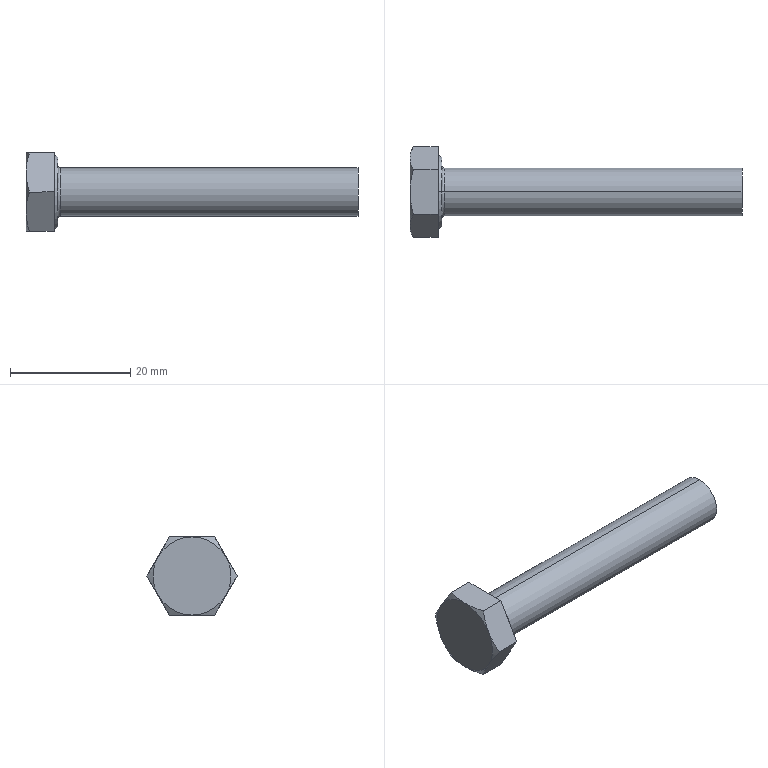Part | SolidWorks | features BaseBody 1, MoveFace 1 | 1 solid | 22 faces | box 55.3 x 15.011 x 13 mm | volume 3267 mm3 | plane 10 | cone 8 | spline 2 | cylinder 2 | commonest cylinder face diameters 8 x2
STEP:
#1=CARTESIAN_POINT('',(5.3,0.,4.4));
#2=VERTEX_POINT('',#1);
#3=CARTESIAN_POINT('',(5.3,0.,-4.4));
#4=VERTEX_POINT('',#3);
#5=CARTESIAN_POINT('',(5.3,0.,4.4));
#6=CARTESIAN_POINT('',(5.3,0.2797,4.4));
#7=CARTESIAN_POINT('',(5.3,0.6919,4.361));
#8=CARTESIAN_POINT('',(5.3,1.16,4.249));
#9=CARTESIAN_POINT('',(5.3,1.391,4.176));
#10=CARTESIAN_POINT('',(5.3,1.489,4.141));
#11=CARTESIAN_POINT('',(5.3,1.554,4.116));
#12=CARTESIAN_POINT('',(5.3,1.585,4.105));
#13=CARTESIAN_POINT('',(5.3,1.758,4.036));
#14=CARTESIAN_POINT('',(5.3,1.96,3.944));
#15=CARTESIAN_POINT('',(5.3,2.154,3.837));
#16=CARTESIAN_POINT('',(5.3,2.282,3.763));
#17=CARTESIAN_POINT('',(5.3,2.344,3.724));
#18=CARTESIAN_POINT('',(5.3,2.662,3.517));
#19=CARTESIAN_POINT('',(5.3,2.897,3.326));
#20=CARTESIAN_POINT('',(5.3,3.219,3.004));
#21=CARTESIAN_POINT('',(5.3,3.37,2.836));
#22=CARTESIAN_POINT('',(5.3,3.509,2.656));
#23=CARTESIAN_POINT('',(5.3,3.598,2.534));
#24=CARTESIAN_POINT('',(5.3,3.642,2.47));
#25=CARTESIAN_POINT('',(5.3,3.764,2.283));
#26=CARTESIAN_POINT('',(5.3,3.876,2.092));
#27=CARTESIAN_POINT('',(5.3,3.989,1.859));
#28=CARTESIAN_POINT('',(5.3,4.042,1.74));
#29=CARTESIAN_POINT('',(5.3,4.063,1.689));
#30=CARTESIAN_POINT('',(5.3,4.077,1.654));
#31=CARTESIAN_POINT('',(5.3,4.085,1.636));
#32=CARTESIAN_POINT('',(5.3,4.297,1.1));
#33=CARTESIAN_POINT('',(5.3,4.4,0.5592));
#34=CARTESIAN_POINT('',(5.3,4.4,-0.2796));
#35=CARTESIAN_POINT('',(5.3,4.361,-0.6917));
#36=CARTESIAN_POINT('',(5.3,4.249,-1.16));
#37=CARTESIAN_POINT('',(5.3,4.176,-1.391));
#38=CARTESIAN_POINT('',(5.3,4.141,-1.489));
#39=CARTESIAN_POINT('',(5.3,4.116,-1.554));
#40=CARTESIAN_POINT('',(5.3,4.105,-1.585));
#41=CARTESIAN_POINT('',(5.3,4.036,-1.758));
#42=CARTESIAN_POINT('',(5.3,3.944,-1.96));
#43=CARTESIAN_POINT('',(5.3,3.837,-2.154));
#44=CARTESIAN_POINT('',(5.3,3.763,-2.282));
#45=CARTESIAN_POINT('',(5.3,3.724,-2.344));
#46=CARTESIAN_POINT('',(5.3,3.517,-2.662));
#47=CARTESIAN_POINT('',(5.3,3.326,-2.897));
#48=CARTESIAN_POINT('',(5.3,3.004,-3.219));
#49=CARTESIAN_POINT('',(5.3,2.836,-3.37));
#50=CARTESIAN_POINT('',(5.3,2.656,-3.509));
#51=CARTESIAN_POINT('',(5.3,2.534,-3.598));
#52=CARTESIAN_POINT('',(5.3,2.47,-3.642));
#53=CARTESIAN_POINT('',(5.3,2.283,-3.764));
#54=CARTESIAN_POINT('',(5.3,2.092,-3.876));
#55=CARTESIAN_POINT('',(5.3,1.859,-3.989));
#56=CARTESIAN_POINT('',(5.3,1.74,-4.042));
#57=CARTESIAN_POINT('',(5.3,1.689,-4.063));
#58=CARTESIAN_POINT('',(5.3,1.654,-4.077));
#59=CARTESIAN_POINT('',(5.3,1.636,-4.085));
#60=CARTESIAN_POINT('',(5.3,1.1,-4.297));
#61=CARTESIAN_POINT('',(5.3,0.5597,-4.4));
#62=CARTESIAN_POINT('',(5.3,0.,-4.4));
#63=B_SPLINE_CURVE_WITH_KNOTS('',3,(#5,#6,#7,#8,#9,#10,#11,#12,#13,#14,#15,#16,#17,#18,#19,#20,#21,#22,#23,#24,#25,#26,#27,#28,#29,#30,#31,#32,#33,#34,#35,#36,#37,#38,#39,#40,#41,#42,#43,#44,#45,#46,#47,#48,#49,#50,#51,#52,#53,#54,#55,#56,#57,#58,#59,#60,#61,#62),.UNSPECIFIED.,.F.,.F.,(4,1,1,1,2,2,1,2,2,2,1,2,2,1,1,1,2,2,2,1,1,1,2,2,1,2,2,2,1,2,2,1,1,1,2,2,4),(0.,0.0625,0.09375,0.1094,0.1172,0.125,0.1563,0.1719,0.1875,0.25,0.2813,0.2969,0.3125,0.3438,0.3594,0.3672,0.3711,0.375,0.5,0.5625,0.5938,0.6094,0.6172,0.625,0.6563,0.6719,0.6875,0.75,0.7813,0.7969,0.8125,0.8438,0.8594,0.8672,0.8711,0.875,1.),.UNSPECIFIED.);
#64=EDGE_CURVE('',#2,#4,#63,.T.);
#65=ORIENTED_EDGE('',*,*,#64,.F.);
#66=CARTESIAN_POINT('',(5.7,0.,4.));
#67=VERTEX_POINT('',#66);
#68=CARTESIAN_POINT('',(5.7,0.,4.4));
#69=DIRECTION('',(0.,-1.,0.));
#70=DIRECTION('',(0.,0.,1.));
#71=AXIS2_PLACEMENT_3D('',#68,#69,#70);
#72=CIRCLE('',#71,0.4);
#73=EDGE_CURVE('',#2,#67,#72,.T.);
#74=ORIENTED_EDGE('',*,*,#73,.T.);
#75=CARTESIAN_POINT('',(5.7,0.,-4.));
#76=VERTEX_POINT('',#75);
#77=CARTESIAN_POINT('',(5.7,0.,0.));
#78=DIRECTION('',(1.,0.,0.));
#79=DIRECTION('',(0.,0.,1.));
#80=AXIS2_PLACEMENT_3D('',#77,#78,#79);
#81=CIRCLE('',#80,4.);
#82=EDGE_CURVE('',#76,#67,#81,.T.);
#83=ORIENTED_EDGE('',*,*,#82,.F.);
#84=CARTESIAN_POINT('',(5.7,0.,-4.4));
#85=DIRECTION('',(0.,1.,0.));
#86=DIRECTION('',(0.,0.,-1.));
#87=AXIS2_PLACEMENT_3D('',#84,#85,#86);
#88=CIRCLE('',#87,0.4);
#89=EDGE_CURVE('',#4,#76,#88,.T.);
#90=ORIENTED_EDGE('',*,*,#89,.F.);
#91=EDGE_LOOP('',(#65,#74,#83,#90));
#92=FACE_OUTER_BOUND('',#91,.T.);
#93=CARTESIAN_POINT('',(5.3,0.,-4.4));
#94=CARTESIAN_POINT('',(5.3,8.8,-4.4));
#95=CARTESIAN_POINT('',(5.3,8.8,4.4));
#96=CARTESIAN_POINT('',(5.3,0.,4.4));
#97=CARTESIAN_POINT('',(5.3,0.,-4.166));
#98=CARTESIAN_POINT('',(5.3,8.331,-4.166));
#99=CARTESIAN_POINT('',(5.3,8.331,4.166));
#100=CARTESIAN_POINT('',(5.3,0.,4.166));
#101=CARTESIAN_POINT('',(5.466,0.,-4.));
#102=CARTESIAN_POINT('',(5.466,8.,-4.));
#103=CARTESIAN_POINT('',(5.466,8.,4.));
#104=CARTESIAN_POINT('',(5.466,0.,4.));
#105=CARTESIAN_POINT('',(5.7,0.,-4.));
#106=CARTESIAN_POINT('',(5.7,8.,-4.));
#107=CARTESIAN_POINT('',(5.7,8.,4.));
#108=CARTESIAN_POINT('',(5.7,0.,4.));
#109=(BOUNDED_SURFACE()B_SPLINE_SURFACE(3,3,((#93,#94,#95,#96),(#97,#98,#99,#100),(#101,#102,#103,#104),(#105,#106,#107,#108)),.UNSPECIFIED.,.F.,.F.,.T.)B_SPLINE_SURFACE_WITH_KNOTS((4,4),(4,4),(0.,1.),(0.,1.),.UNSPECIFIED.)GEOMETRIC_REPRESENTATION_ITEM()RATIONAL_B_SPLINE_SURFACE(((1.,0.3333,0.3333,1.),(0.8047,0.2682,0.2682,0.8047),(0.8047,0.2682,0.2682,0.8047),(1.,0.3333,0.3333,1.)))REPRESENTATION_ITEM('')SURFACE());
#110=ADVANCED_FACE('',(#92),#109,.F.);
#111=CARTESIAN_POINT('',(55.3,0.,4.));
#112=VERTEX_POINT('',#111);
#113=CARTESIAN_POINT('',(55.3,0.,-4.));
#114=VERTEX_POINT('',#113);
#115=CARTESIAN_POINT('',(55.3,0.,0.));
#116=DIRECTION('',(-1.,0.,0.));
#117=DIRECTION('',(0.,0.,1.));
#118=AXIS2_PLACEMENT_3D('',#115,#116,#117);
#119=CIRCLE('',#118,4.);
#120=EDGE_CURVE('',#112,#114,#119,.T.);
#121=ORIENTED_EDGE('',*,*,#120,.T.);
#122=CARTESIAN_POINT('',(0.,0.,-4.));
#123=DIRECTION('',(-1.,0.,0.));
#124=VECTOR('',#123,1000.);
#125=LINE('',#122,#124);
#126=EDGE_CURVE('',#114,#76,#125,.T.);
#127=ORIENTED_EDGE('',*,*,#126,.T.);
#128=ORIENTED_EDGE('',*,*,#82,.T.);
#129=CARTESIAN_POINT('',(0.,0.,4.));
#130=DIRECTION('',(-1.,0.,0.));
#131=VECTOR('',#130,1000.);
#132=LINE('',#129,#131);
#133=EDGE_CURVE('',#112,#67,#132,.T.);
#134=ORIENTED_EDGE('',*,*,#133,.F.);
#135=EDGE_LOOP('',(#121,#127,#128,#134));
#136=FACE_OUTER_BOUND('',#135,.T.);
#137=CARTESIAN_POINT('',(0.,0.,0.));
#138=DIRECTION('',(-1.,0.,0.));
#139=DIRECTION('',(0.,0.,1.));
#140=AXIS2_PLACEMENT_3D('',#137,#138,#139);
#141=CYLINDRICAL_SURFACE('',#140,4.);
#142=ADVANCED_FACE('',(#136),#141,.T.);
#143=CARTESIAN_POINT('',(5.3,0.,-5.815));
#144=VERTEX_POINT('',#143);
#145=CARTESIAN_POINT('',(5.3,0.,5.815));
#146=VERTEX_POINT('',#145);
#147=CARTESIAN_POINT('',(5.3,0.,0.));
#148=DIRECTION('',(1.,0.,0.));
#149=DIRECTION('',(0.,0.,1.));
#150=AXIS2_PLACEMENT_3D('',#147,#148,#149);
#151=CIRCLE('',#150,5.815);
#152=EDGE_CURVE('',#144,#146,#151,.T.);
#153=ORIENTED_EDGE('',*,*,#152,.F.);
#154=CARTESIAN_POINT('',(4.7,0.,-6.161));
#155=VERTEX_POINT('',#154);
#156=CARTESIAN_POINT('',(4.7,0.,-6.161));
#157=DIRECTION('',(-0.866,0.,-0.5));
#158=VECTOR('',#157,1000.);
#159=LINE('',#156,#158);
#160=EDGE_CURVE('',#144,#155,#159,.T.);
#161=ORIENTED_EDGE('',*,*,#160,.T.);
#162=CARTESIAN_POINT('',(4.7,0.,6.161));
#163=VERTEX_POINT('',#162);
#164=CARTESIAN_POINT('',(4.7,0.,0.));
#165=DIRECTION('',(1.,0.,0.));
#166=DIRECTION('',(0.,0.,1.));
#167=AXIS2_PLACEMENT_3D('',#164,#165,#166);
#168=CIRCLE('',#167,6.161);
#169=EDGE_CURVE('',#155,#163,#168,.T.);
#170=ORIENTED_EDGE('',*,*,#169,.T.);
#171=CARTESIAN_POINT('',(4.7,0.,6.161));
#172=DIRECTION('',(-0.866,0.,0.5));
#173=VECTOR('',#172,1000.);
#174=LINE('',#171,#173);
#175=EDGE_CURVE('',#146,#163,#174,.T.);
#176=ORIENTED_EDGE('',*,*,#175,.F.);
#177=EDGE_LOOP('',(#153,#161,#170,#176));
#178=FACE_OUTER_BOUND('',#177,.T.);
#179=CARTESIAN_POINT('',(4.7,0.,0.));
#180=DIRECTION('',(-1.,0.,0.));
#181=DIRECTION('',(0.,0.,1.));
#182=AXIS2_PLACEMENT_3D('',#179,#180,#181);
#183=CONICAL_SURFACE('',#182,6.161,0.5236);
#184=ADVANCED_FACE('',(#178),#183,.T.);
#185=ORIENTED_EDGE('',*,*,#126,.F.);
#186=CARTESIAN_POINT('',(55.3,0.,0.));
#187=DIRECTION('',(-1.,0.,0.));
#188=DIRECTION('',(0.,0.,1.));
#189=AXIS2_PLACEMENT_3D('',#186,#187,#188);
#190=CIRCLE('',#189,4.);
#191=EDGE_CURVE('',#114,#112,#190,.T.);
#192=ORIENTED_EDGE('',*,*,#191,.T.);
#193=ORIENTED_EDGE('',*,*,#133,.T.);
#194=CARTESIAN_POINT('',(5.7,0.,0.));
#195=DIRECTION('',(1.,0.,0.));
#196=DIRECTION('',(0.,0.,1.));
#197=AXIS2_PLACEMENT_3D('',#194,#195,#196);
#198=CIRCLE('',#197,4.);
#199=EDGE_CURVE('',#67,#76,#198,.T.);
#200=ORIENTED_EDGE('',*,*,#199,.T.);
#201=EDGE_LOOP('',(#185,#192,#193,#200));
#202=FACE_OUTER_BOUND('',#201,.T.);
#203=CARTESIAN_POINT('',(0.,0.,0.));
#204=DIRECTION('',(-1.,0.,0.));
#205=DIRECTION('',(0.,0.,1.));
#206=AXIS2_PLACEMENT_3D('',#203,#204,#205);
#207=CYLINDRICAL_SURFACE('',#206,4.);
#208=ADVANCED_FACE('',(#202),#207,.T.);
#209=ORIENTED_EDGE('',*,*,#73,.F.);
#210=CARTESIAN_POINT('',(5.3,0.,-4.4));
#211=CARTESIAN_POINT('',(5.3,-0.2797,-4.4));
#212=CARTESIAN_POINT('',(5.3,-0.6919,-4.361));
#213=CARTESIAN_POINT('',(5.3,-1.16,-4.249));
#214=CARTESIAN_POINT('',(5.3,-1.391,-4.176));
#215=CARTESIAN_POINT('',(5.3,-1.489,-4.141));
#216=CARTESIAN_POINT('',(5.3,-1.554,-4.116));
#217=CARTESIAN_POINT('',(5.3,-1.585,-4.105));
#218=CARTESIAN_POINT('',(5.3,-1.758,-4.036));
#219=CARTESIAN_POINT('',(5.3,-1.96,-3.944));
#220=CARTESIAN_POINT('',(5.3,-2.154,-3.837));
#221=CARTESIAN_POINT('',(5.3,-2.282,-3.763));
#222=CARTESIAN_POINT('',(5.3,-2.344,-3.724));
#223=CARTESIAN_POINT('',(5.3,-2.662,-3.517));
#224=CARTESIAN_POINT('',(5.3,-2.897,-3.326));
#225=CARTESIAN_POINT('',(5.3,-3.219,-3.004));
#226=CARTESIAN_POINT('',(5.3,-3.37,-2.836));
#227=CARTESIAN_POINT('',(5.3,-3.509,-2.656));
#228=CARTESIAN_POINT('',(5.3,-3.598,-2.534));
#229=CARTESIAN_POINT('',(5.3,-3.642,-2.47));
#230=CARTESIAN_POINT('',(5.3,-3.764,-2.283));
#231=CARTESIAN_POINT('',(5.3,-3.876,-2.092));
#232=CARTESIAN_POINT('',(5.3,-3.989,-1.859));
#233=CARTESIAN_POINT('',(5.3,-4.042,-1.74));
#234=CARTESIAN_POINT('',(5.3,-4.063,-1.689));
#235=CARTESIAN_POINT('',(5.3,-4.077,-1.654));
#236=CARTESIAN_POINT('',(5.3,-4.085,-1.636));
#237=CARTESIAN_POINT('',(5.3,-4.297,-1.1));
#238=CARTESIAN_POINT('',(5.3,-4.4,-0.5592));
#239=CARTESIAN_POINT('',(5.3,-4.4,0.2796));
#240=CARTESIAN_POINT('',(5.3,-4.361,0.6917));
#241=CARTESIAN_POINT('',(5.3,-4.249,1.16));
#242=CARTESIAN_POINT('',(5.3,-4.176,1.391));
#243=CARTESIAN_POINT('',(5.3,-4.141,1.489));
#244=CARTESIAN_POINT('',(5.3,-4.116,1.554));
#245=CARTESIAN_POINT('',(5.3,-4.105,1.585));
#246=CARTESIAN_POINT('',(5.3,-4.036,1.758));
#247=CARTESIAN_POINT('',(5.3,-3.944,1.96));
#248=CARTESIAN_POINT('',(5.3,-3.837,2.154));
#249=CARTESIAN_POINT('',(5.3,-3.763,2.282));
#250=CARTESIAN_POINT('',(5.3,-3.724,2.344));
#251=CARTESIAN_POINT('',(5.3,-3.517,2.662));
#252=CARTESIAN_POINT('',(5.3,-3.326,2.897));
#253=CARTESIAN_POINT('',(5.3,-3.004,3.219));
#254=CARTESIAN_POINT('',(5.3,-2.836,3.37));
#255=CARTESIAN_POINT('',(5.3,-2.656,3.509));
#256=CARTESIAN_POINT('',(5.3,-2.534,3.598));
#257=CARTESIAN_POINT('',(5.3,-2.47,3.642));
#258=CARTESIAN_POINT('',(5.3,-2.283,3.764));
#259=CARTESIAN_POINT('',(5.3,-2.092,3.876));
#260=CARTESIAN_POINT('',(5.3,-1.859,3.989));
#261=CARTESIAN_POINT('',(5.3,-1.74,4.042));
#262=CARTESIAN_POINT('',(5.3,-1.689,4.063));
#263=CARTESIAN_POINT('',(5.3,-1.654,4.077));
#264=CARTESIAN_POINT('',(5.3,-1.636,4.085));
#265=CARTESIAN_POINT('',(5.3,-1.1,4.297));
#266=CARTESIAN_POINT('',(5.3,-0.5597,4.4));
#267=CARTESIAN_POINT('',(5.3,0.,4.4));
#268=B_SPLINE_CURVE_WITH_KNOTS('',3,(#210,#211,#212,#213,#214,#215,#216,#217,#218,#219,#220,#221,#222,#223,#224,#225,#226,#227,#228,#229,#230,#231,#232,#233,#234,#235,#236,#237,#238,#239,#240,#241,#242,#243,#244,#245,#246,#247,#248,#249,#250,#251,#252,#253,#254,#255,#256,#257,#258,#259,#260,#261,#262,#263,#264,#265,#266,#267),.UNSPECIFIED.,.F.,.F.,(4,1,1,1,2,2,1,2,2,2,1,2,2,1,1,1,2,2,2,1,1,1,2,2,1,2,2,2,1,2,2,1,1,1,2,2,4),(0.,0.0625,0.09375,0.1094,0.1172,0.125,0.1563,0.1719,0.1875,0.25,0.2813,0.2969,0.3125,0.3437,0.3594,0.3672,0.3711,0.375,0.5,0.5625,0.5938,0.6094,0.6172,0.625,0.6563,0.6719,0.6875,0.75,0.7813,0.7969,0.8125,0.8437,0.8594,0.8672,0.8711,0.875,1.),.UNSPECIFIED.);
#269=EDGE_CURVE('',#4,#2,#268,.T.);
#270=ORIENTED_EDGE('',*,*,#269,.F.);
#271=ORIENTED_EDGE('',*,*,#89,.T.);
#272=ORIENTED_EDGE('',*,*,#199,.F.);
#273=EDGE_LOOP('',(#209,#270,#271,#272));
#274=FACE_OUTER_BOUND('',#273,.T.);
#275=CARTESIAN_POINT('',(5.3,0.,4.4));
#276=CARTESIAN_POINT('',(5.3,-8.8,4.4));
#277=CARTESIAN_POINT('',(5.3,-8.8,-4.4));
#278=CARTESIAN_POINT('',(5.3,0.,-4.4));
#279=CARTESIAN_POINT('',(5.3,0.,4.166));
#280=CARTESIAN_POINT('',(5.3,-8.331,4.166));
#281=CARTESIAN_POINT('',(5.3,-8.331,-4.166));
#282=CARTESIAN_POINT('',(5.3,0.,-4.166));
#283=CARTESIAN_POINT('',(5.466,0.,4.));
#284=CARTESIAN_POINT('',(5.466,-8.,4.));
#285=CARTESIAN_POINT('',(5.466,-8.,-4.));
#286=CARTESIAN_POINT('',(5.466,0.,-4.));
#287=CARTESIAN_POINT('',(5.7,0.,4.));
#288=CARTESIAN_POINT('',(5.7,-8.,4.));
#289=CARTESIAN_POINT('',(5.7,-8.,-4.));
#290=CARTESIAN_POINT('',(5.7,0.,-4.));
#291=(BOUNDED_SURFACE()B_SPLINE_SURFACE(3,3,((#275,#276,#277,#278),(#279,#280,#281,#282),(#283,#284,#285,#286),(#287,#288,#289,#290)),.UNSPECIFIED.,.F.,.F.,.T.)B_SPLINE_SURFACE_WITH_KNOTS((4,4),(4,4),(0.,1.),(0.,1.),.UNSPECIFIED.)GEOMETRIC_REPRESENTATION_ITEM()RATIONAL_B_SPLINE_SURFACE(((1.,0.3333,0.3333,1.),(0.8047,0.2682,0.2682,0.8047),(0.8047,0.2682,0.2682,0.8047),(1.,0.3333,0.3333,1.)))REPRESENTATION_ITEM('')SURFACE());
#292=ADVANCED_FACE('',(#274),#291,.F.);
#293=ORIENTED_EDGE('',*,*,#120,.F.);
#294=ORIENTED_EDGE('',*,*,#191,.F.);
#295=EDGE_LOOP('',(#293,#294));
#296=FACE_OUTER_BOUND('',#295,.T.);
#297=CARTESIAN_POINT('',(55.3,0.,0.));
#298=DIRECTION('',(-1.,0.,0.));
#299=DIRECTION('',(0.,0.,1.));
#300=AXIS2_PLACEMENT_3D('',#297,#298,#299);
#301=PLANE('',#300);
#302=ADVANCED_FACE('',(#296),#301,.F.);
#303=CARTESIAN_POINT('',(5.3,0.,0.));
#304=DIRECTION('',(1.,0.,0.));
#305=DIRECTION('',(0.,0.,1.));
#306=AXIS2_PLACEMENT_3D('',#303,#304,#305);
#307=CIRCLE('',#306,5.815);
#308=EDGE_CURVE('',#146,#144,#307,.T.);
#309=ORIENTED_EDGE('',*,*,#308,.T.);
#310=ORIENTED_EDGE('',*,*,#152,.T.);
#311=EDGE_LOOP('',(#309,#310));
#312=FACE_OUTER_BOUND('',#311,.T.);
#313=ORIENTED_EDGE('',*,*,#269,.T.);
#314=ORIENTED_EDGE('',*,*,#64,.T.);
#315=EDGE_LOOP('',(#313,#314));
#316=FACE_BOUND('',#315,.T.);
#317=CARTESIAN_POINT('',(5.3,7.506,0.));
#318=DIRECTION('',(1.,0.,0.));
#319=DIRECTION('',(0.,0.,-1.));
#320=AXIS2_PLACEMENT_3D('',#317,#318,#319);
#321=PLANE('',#320);
#322=ADVANCED_FACE('',(#312,#316),#321,.T.);
#323=ORIENTED_EDGE('',*,*,#160,.F.);
#324=ORIENTED_EDGE('',*,*,#308,.F.);
#325=ORIENTED_EDGE('',*,*,#175,.T.);
#326=CARTESIAN_POINT('',(4.7,0.,0.));
#327=DIRECTION('',(1.,0.,0.));
#328=DIRECTION('',(0.,0.,1.));
#329=AXIS2_PLACEMENT_3D('',#326,#327,#328);
#330=CIRCLE('',#329,6.161);
#331=EDGE_CURVE('',#163,#155,#330,.T.);
#332=ORIENTED_EDGE('',*,*,#331,.T.);
#333=EDGE_LOOP('',(#323,#324,#325,#332));
#334=FACE_OUTER_BOUND('',#333,.T.);
#335=CARTESIAN_POINT('',(4.7,0.,0.));
#336=DIRECTION('',(-1.,0.,0.));
#337=DIRECTION('',(0.,0.,1.));
#338=AXIS2_PLACEMENT_3D('',#335,#336,#337);
#339=CONICAL_SURFACE('',#338,6.161,0.5236);
#340=ADVANCED_FACE('',(#334),#339,.T.);
#341=CARTESIAN_POINT('',(4.7,-7.506,0.));
#342=VERTEX_POINT('',#341);
#343=CARTESIAN_POINT('',(4.7,-3.753,-6.5));
#344=VERTEX_POINT('',#343);
#345=CARTESIAN_POINT('',(4.7,-7.506,0.));
#346=DIRECTION('',(0.,0.5,-0.866));
#347=VECTOR('',#346,1000.);
#348=LINE('',#345,#347);
#349=EDGE_CURVE('',#342,#344,#348,.T.);
#350=ORIENTED_EDGE('',*,*,#349,.T.);
#351=CARTESIAN_POINT('',(4.7,3.753,-6.5));
#352=VERTEX_POINT('',#351);
#353=CARTESIAN_POINT('',(4.7,6.161,-6.5));
#354=DIRECTION('',(0.,1.,0.));
#355=VECTOR('',#354,1000.);
#356=LINE('',#353,#355);
#357=EDGE_CURVE('',#344,#352,#356,.T.);
#358=ORIENTED_EDGE('',*,*,#357,.T.);
#359=CARTESIAN_POINT('',(4.7,7.506,0.));
#360=VERTEX_POINT('',#359);
#361=CARTESIAN_POINT('',(4.7,3.753,-6.5));
#362=DIRECTION('',(0.,0.5,0.866));
#363=VECTOR('',#362,1000.);
#364=LINE('',#361,#363);
#365=EDGE_CURVE('',#352,#360,#364,.T.);
#366=ORIENTED_EDGE('',*,*,#365,.T.);
#367=CARTESIAN_POINT('',(4.7,3.753,6.5));
#368=VERTEX_POINT('',#367);
#369=CARTESIAN_POINT('',(4.7,7.506,0.));
#370=DIRECTION('',(0.,-0.5,0.866));
#371=VECTOR('',#370,1000.);
#372=LINE('',#369,#371);
#373=EDGE_CURVE('',#360,#368,#372,.T.);
#374=ORIENTED_EDGE('',*,*,#373,.T.);
#375=CARTESIAN_POINT('',(4.7,-3.753,6.5));
#376=VERTEX_POINT('',#375);
#377=CARTESIAN_POINT('',(4.7,6.161,6.5));
#378=DIRECTION('',(0.,-1.,0.));
#379=VECTOR('',#378,1000.);
#380=LINE('',#377,#379);
#381=EDGE_CURVE('',#368,#376,#380,.T.);
#382=ORIENTED_EDGE('',*,*,#381,.T.);
#383=CARTESIAN_POINT('',(4.7,-3.753,6.5));
#384=DIRECTION('',(0.,-0.5,-0.866));
#385=VECTOR('',#384,1000.);
#386=LINE('',#383,#385);
#387=EDGE_CURVE('',#376,#342,#386,.T.);
#388=ORIENTED_EDGE('',*,*,#387,.T.);
#389=EDGE_LOOP('',(#350,#358,#366,#374,#382,#388));
#390=FACE_OUTER_BOUND('',#389,.T.);
#391=ORIENTED_EDGE('',*,*,#331,.F.);
#392=ORIENTED_EDGE('',*,*,#169,.F.);
#393=EDGE_LOOP('',(#391,#392));
#394=FACE_BOUND('',#393,.T.);
#395=CARTESIAN_POINT('',(4.7,6.161,0.));
#396=DIRECTION('',(1.,0.,0.));
#397=DIRECTION('',(0.,0.,-1.));
#398=AXIS2_PLACEMENT_3D('',#395,#396,#397);
#399=PLANE('',#398);
#400=ADVANCED_FACE('',(#390,#394),#399,.T.);
#401=CARTESIAN_POINT('',(0.5806,-3.753,-6.5));
#402=VERTEX_POINT('',#401);
#403=CARTESIAN_POINT('',(5.3,-3.753,-6.5));
#404=DIRECTION('',(1.,0.,0.));
#405=VECTOR('',#404,1000.);
#406=LINE('',#403,#405);
#407=EDGE_CURVE('',#402,#344,#406,.T.);
#408=ORIENTED_EDGE('',*,*,#407,.F.);
#409=CARTESIAN_POINT('',(0.,0.,-6.5));
#410=VERTEX_POINT('',#409);
#411=CARTESIAN_POINT('',(0.,0.,-6.5));
#412=CARTESIAN_POINT('',(0.,-1.281,-6.5));
#413=CARTESIAN_POINT('',(0.2266,-2.527,-6.5));
#414=CARTESIAN_POINT('',(0.5806,-3.753,-6.5));
#415=B_SPLINE_CURVE_WITH_KNOTS('',3,(#411,#412,#413,#414),.UNSPECIFIED.,.F.,.F.,(4,4),(0.,0.003797),.UNSPECIFIED.);
#416=EDGE_CURVE('',#410,#402,#415,.T.);
#417=ORIENTED_EDGE('',*,*,#416,.F.);
#418=CARTESIAN_POINT('',(0.5806,3.753,-6.5));
#419=VERTEX_POINT('',#418);
#420=CARTESIAN_POINT('',(0.5806,3.753,-6.5));
#421=CARTESIAN_POINT('',(0.2266,2.527,-6.5));
#422=CARTESIAN_POINT('',(0.,1.281,-6.5));
#423=CARTESIAN_POINT('',(0.,0.,-6.5));
#424=B_SPLINE_CURVE_WITH_KNOTS('',3,(#420,#421,#422,#423),.UNSPECIFIED.,.F.,.F.,(4,4),(0.,0.003797),.UNSPECIFIED.);
#425=EDGE_CURVE('',#419,#410,#424,.T.);
#426=ORIENTED_EDGE('',*,*,#425,.F.);
#427=CARTESIAN_POINT('',(5.3,3.753,-6.5));
#428=DIRECTION('',(-1.,0.,0.));
#429=VECTOR('',#428,1000.);
#430=LINE('',#427,#429);
#431=EDGE_CURVE('',#352,#419,#430,.T.);
#432=ORIENTED_EDGE('',*,*,#431,.F.);
#433=ORIENTED_EDGE('',*,*,#357,.F.);
#434=EDGE_LOOP('',(#408,#417,#426,#432,#433));
#435=FACE_OUTER_BOUND('',#434,.T.);
#436=CARTESIAN_POINT('',(5.3,3.753,-6.5));
#437=DIRECTION('',(0.,0.,1.));
#438=DIRECTION('',(0.,-1.,0.));
#439=AXIS2_PLACEMENT_3D('',#436,#437,#438);
#440=PLANE('',#439);
#441=ADVANCED_FACE('',(#435),#440,.F.);
#442=CARTESIAN_POINT('',(0.5806,-7.506,0.));
#443=VERTEX_POINT('',#442);
#444=CARTESIAN_POINT('',(5.3,-7.506,0.));
#445=DIRECTION('',(1.,0.,0.));
#446=VECTOR('',#445,1000.);
#447=LINE('',#444,#446);
#448=EDGE_CURVE('',#443,#342,#447,.T.);
#449=ORIENTED_EDGE('',*,*,#448,.F.);
#450=CARTESIAN_POINT('',(0.,-5.629,-3.25));
#451=VERTEX_POINT('',#450);
#452=CARTESIAN_POINT('',(0.,-5.629,-3.25));
#453=CARTESIAN_POINT('',(0.,-6.27,-2.141));
#454=CARTESIAN_POINT('',(0.2266,-6.892,-1.062));
#455=CARTESIAN_POINT('',(0.5806,-7.506,0.));
#456=B_SPLINE_CURVE_WITH_KNOTS('',3,(#452,#453,#454,#455),.UNSPECIFIED.,.F.,.F.,(4,4),(0.,0.003797),.UNSPECIFIED.);
#457=EDGE_CURVE('',#451,#443,#456,.T.);
#458=ORIENTED_EDGE('',*,*,#457,.F.);
#459=CARTESIAN_POINT('',(0.5806,-3.753,-6.5));
#460=CARTESIAN_POINT('',(0.2266,-4.366,-5.438));
#461=CARTESIAN_POINT('',(0.,-4.989,-4.359));
#462=CARTESIAN_POINT('',(0.,-5.629,-3.25));
#463=B_SPLINE_CURVE_WITH_KNOTS('',3,(#459,#460,#461,#462),.UNSPECIFIED.,.F.,.F.,(4,4),(0.,0.003797),.UNSPECIFIED.);
#464=EDGE_CURVE('',#402,#451,#463,.T.);
#465=ORIENTED_EDGE('',*,*,#464,.F.);
#466=ORIENTED_EDGE('',*,*,#407,.T.);
#467=ORIENTED_EDGE('',*,*,#349,.F.);
#468=EDGE_LOOP('',(#449,#458,#465,#466,#467));
#469=FACE_OUTER_BOUND('',#468,.T.);
#470=CARTESIAN_POINT('',(5.3,-3.753,-6.5));
#471=DIRECTION('',(0.,0.866,0.5));
#472=DIRECTION('',(0.,-0.5,0.866));
#473=AXIS2_PLACEMENT_3D('',#470,#471,#472);
#474=PLANE('',#473);
#475=ADVANCED_FACE('',(#469),#474,.F.);
#476=CARTESIAN_POINT('',(0.5806,-3.753,6.5));
#477=VERTEX_POINT('',#476);
#478=CARTESIAN_POINT('',(5.3,-3.753,6.5));
#479=DIRECTION('',(1.,0.,0.));
#480=VECTOR('',#479,1000.);
#481=LINE('',#478,#480);
#482=EDGE_CURVE('',#477,#376,#481,.T.);
#483=ORIENTED_EDGE('',*,*,#482,.F.);
#484=CARTESIAN_POINT('',(0.,-5.629,3.25));
#485=VERTEX_POINT('',#484);
#486=CARTESIAN_POINT('',(0.,-5.629,3.25));
#487=CARTESIAN_POINT('',(0.,-4.989,4.359));
#488=CARTESIAN_POINT('',(0.2266,-4.366,5.438));
#489=CARTESIAN_POINT('',(0.5806,-3.753,6.5));
#490=B_SPLINE_CURVE_WITH_KNOTS('',3,(#486,#487,#488,#489),.UNSPECIFIED.,.F.,.F.,(4,4),(0.,0.003797),.UNSPECIFIED.);
#491=EDGE_CURVE('',#485,#477,#490,.T.);
#492=ORIENTED_EDGE('',*,*,#491,.F.);
#493=CARTESIAN_POINT('',(0.5806,-7.506,0.));
#494=CARTESIAN_POINT('',(0.2266,-6.892,1.062));
#495=CARTESIAN_POINT('',(0.,-6.27,2.141));
#496=CARTESIAN_POINT('',(0.,-5.629,3.25));
#497=B_SPLINE_CURVE_WITH_KNOTS('',3,(#493,#494,#495,#496),.UNSPECIFIED.,.F.,.F.,(4,4),(0.,0.003797),.UNSPECIFIED.);
#498=EDGE_CURVE('',#443,#485,#497,.T.);
#499=ORIENTED_EDGE('',*,*,#498,.F.);
#500=ORIENTED_EDGE('',*,*,#448,.T.);
#501=ORIENTED_EDGE('',*,*,#387,.F.);
#502=EDGE_LOOP('',(#483,#492,#499,#500,#501));
#503=FACE_OUTER_BOUND('',#502,.T.);
#504=CARTESIAN_POINT('',(5.3,-7.506,0.));
#505=DIRECTION('',(0.,0.866,-0.5));
#506=DIRECTION('',(0.,0.5,0.866));
#507=AXIS2_PLACEMENT_3D('',#504,#505,#506);
#508=PLANE('',#507);
#509=ADVANCED_FACE('',(#503),#508,.F.);
#510=CARTESIAN_POINT('',(0.5806,3.753,6.5));
#511=VERTEX_POINT('',#510);
#512=CARTESIAN_POINT('',(5.3,3.753,6.5));
#513=DIRECTION('',(1.,0.,0.));
#514=VECTOR('',#513,1000.);
#515=LINE('',#512,#514);
#516=EDGE_CURVE('',#511,#368,#515,.T.);
#517=ORIENTED_EDGE('',*,*,#516,.F.);
#518=CARTESIAN_POINT('',(0.,0.,6.5));
#519=VERTEX_POINT('',#518);
#520=CARTESIAN_POINT('',(0.,0.,6.5));
#521=CARTESIAN_POINT('',(0.,1.281,6.5));
#522=CARTESIAN_POINT('',(0.2266,2.527,6.5));
#523=CARTESIAN_POINT('',(0.5806,3.753,6.5));
#524=B_SPLINE_CURVE_WITH_KNOTS('',3,(#520,#521,#522,#523),.UNSPECIFIED.,.F.,.F.,(4,4),(0.,0.003797),.UNSPECIFIED.);
#525=EDGE_CURVE('',#519,#511,#524,.T.);
#526=ORIENTED_EDGE('',*,*,#525,.F.);
#527=CARTESIAN_POINT('',(0.5806,-3.753,6.5));
#528=CARTESIAN_POINT('',(0.2266,-2.527,6.5));
#529=CARTESIAN_POINT('',(0.,-1.281,6.5));
#530=CARTESIAN_POINT('',(0.,0.,6.5));
#531=B_SPLINE_CURVE_WITH_KNOTS('',3,(#527,#528,#529,#530),.UNSPECIFIED.,.F.,.F.,(4,4),(0.,0.003797),.UNSPECIFIED.);
#532=EDGE_CURVE('',#477,#519,#531,.T.);
#533=ORIENTED_EDGE('',*,*,#532,.F.);
#534=ORIENTED_EDGE('',*,*,#482,.T.);
#535=ORIENTED_EDGE('',*,*,#381,.F.);
#536=EDGE_LOOP('',(#517,#526,#533,#534,#535));
#537=FACE_OUTER_BOUND('',#536,.T.);
#538=CARTESIAN_POINT('',(5.3,3.753,6.5));
#539=DIRECTION('',(0.,0.,-1.));
#540=DIRECTION('',(0.,1.,0.));
#541=AXIS2_PLACEMENT_3D('',#538,#539,#540);
#542=PLANE('',#541);
#543=ADVANCED_FACE('',(#537),#542,.F.);
#544=CARTESIAN_POINT('',(0.5806,7.506,0.));
#545=VERTEX_POINT('',#544);
#546=CARTESIAN_POINT('',(5.3,7.506,0.));
#547=DIRECTION('',(1.,0.,0.));
#548=VECTOR('',#547,1000.);
#549=LINE('',#546,#548);
#550=EDGE_CURVE('',#545,#360,#549,.T.);
#551=ORIENTED_EDGE('',*,*,#550,.F.);
#552=CARTESIAN_POINT('',(0.,5.629,3.25));
#553=VERTEX_POINT('',#552);
#554=CARTESIAN_POINT('',(0.,5.629,3.25));
#555=CARTESIAN_POINT('',(0.,6.27,2.141));
#556=CARTESIAN_POINT('',(0.2266,6.892,1.062));
#557=CARTESIAN_POINT('',(0.5806,7.506,0.));
#558=B_SPLINE_CURVE_WITH_KNOTS('',3,(#554,#555,#556,#557),.UNSPECIFIED.,.F.,.F.,(4,4),(0.,0.003797),.UNSPECIFIED.);
#559=EDGE_CURVE('',#553,#545,#558,.T.);
#560=ORIENTED_EDGE('',*,*,#559,.F.);
#561=CARTESIAN_POINT('',(0.5806,3.753,6.5));
#562=CARTESIAN_POINT('',(0.2266,4.366,5.438));
#563=CARTESIAN_POINT('',(0.,4.989,4.359));
#564=CARTESIAN_POINT('',(0.,5.629,3.25));
#565=B_SPLINE_CURVE_WITH_KNOTS('',3,(#561,#562,#563,#564),.UNSPECIFIED.,.F.,.F.,(4,4),(0.,0.003797),.UNSPECIFIED.);
#566=EDGE_CURVE('',#511,#553,#565,.T.);
#567=ORIENTED_EDGE('',*,*,#566,.F.);
#568=ORIENTED_EDGE('',*,*,#516,.T.);
#569=ORIENTED_EDGE('',*,*,#373,.F.);
#570=EDGE_LOOP('',(#551,#560,#567,#568,#569));
#571=FACE_OUTER_BOUND('',#570,.T.);
#572=CARTESIAN_POINT('',(5.3,7.506,0.));
#573=DIRECTION('',(0.,-0.866,-0.5));
#574=DIRECTION('',(0.,0.5,-0.866));
#575=AXIS2_PLACEMENT_3D('',#572,#573,#574);
#576=PLANE('',#575);
#577=ADVANCED_FACE('',(#571),#576,.F.);
#578=ORIENTED_EDGE('',*,*,#431,.T.);
#579=CARTESIAN_POINT('',(0.,5.629,-3.25));
#580=VERTEX_POINT('',#579);
#581=CARTESIAN_POINT('',(0.,5.629,-3.25));
#582=CARTESIAN_POINT('',(0.,4.989,-4.359));
#583=CARTESIAN_POINT('',(0.2266,4.366,-5.438));
#584=CARTESIAN_POINT('',(0.5806,3.753,-6.5));
#585=B_SPLINE_CURVE_WITH_KNOTS('',3,(#581,#582,#583,#584),.UNSPECIFIED.,.F.,.F.,(4,4),(0.,0.003797),.UNSPECIFIED.);
#586=EDGE_CURVE('',#580,#419,#585,.T.);
#587=ORIENTED_EDGE('',*,*,#586,.F.);
#588=CARTESIAN_POINT('',(0.5806,7.506,0.));
#589=CARTESIAN_POINT('',(0.2266,6.892,-1.062));
#590=CARTESIAN_POINT('',(0.,6.27,-2.141));
#591=CARTESIAN_POINT('',(0.,5.629,-3.25));
#592=B_SPLINE_CURVE_WITH_KNOTS('',3,(#588,#589,#590,#591),.UNSPECIFIED.,.F.,.F.,(4,4),(0.,0.003797),.UNSPECIFIED.);
#593=EDGE_CURVE('',#545,#580,#592,.T.);
#594=ORIENTED_EDGE('',*,*,#593,.F.);
#595=ORIENTED_EDGE('',*,*,#550,.T.);
#596=ORIENTED_EDGE('',*,*,#365,.F.);
#597=EDGE_LOOP('',(#578,#587,#594,#595,#596));
#598=FACE_OUTER_BOUND('',#597,.T.);
#599=CARTESIAN_POINT('',(5.3,3.753,-6.5));
#600=DIRECTION('',(0.,-0.866,0.5));
#601=DIRECTION('',(0.,-0.5,-0.866));
#602=AXIS2_PLACEMENT_3D('',#599,#600,#601);
#603=PLANE('',#602);
#604=ADVANCED_FACE('',(#598),#603,.F.);
#605=CARTESIAN_POINT('',(0.,0.,0.));
#606=DIRECTION('',(1.,0.,0.));
#607=DIRECTION('',(0.,0.,-1.));
#608=AXIS2_PLACEMENT_3D('',#605,#606,#607);
#609=CIRCLE('',#608,6.5);
#610=EDGE_CURVE('',#451,#410,#609,.T.);
#611=ORIENTED_EDGE('',*,*,#610,.T.);
#612=ORIENTED_EDGE('',*,*,#416,.T.);
#613=ORIENTED_EDGE('',*,*,#464,.T.);
#614=EDGE_LOOP('',(#611,#612,#613));
#615=FACE_OUTER_BOUND('',#614,.T.);
#616=CARTESIAN_POINT('',(0.584,0.,0.));
#617=DIRECTION('',(1.,0.,0.));
#618=DIRECTION('',(0.,0.,-1.));
#619=AXIS2_PLACEMENT_3D('',#616,#617,#618);
#620=CONICAL_SURFACE('',#619,7.512,1.047);
#621=ADVANCED_FACE('',(#615),#620,.T.);
#622=ORIENTED_EDGE('',*,*,#425,.T.);
#623=CARTESIAN_POINT('',(0.,0.,0.));
#624=DIRECTION('',(1.,0.,0.));
#625=DIRECTION('',(0.,0.,-1.));
#626=AXIS2_PLACEMENT_3D('',#623,#624,#625);
#627=CIRCLE('',#626,6.5);
#628=EDGE_CURVE('',#410,#580,#627,.T.);
#629=ORIENTED_EDGE('',*,*,#628,.T.);
#630=ORIENTED_EDGE('',*,*,#586,.T.);
#631=EDGE_LOOP('',(#622,#629,#630));
#632=FACE_OUTER_BOUND('',#631,.T.);
#633=CARTESIAN_POINT('',(0.584,0.,0.));
#634=DIRECTION('',(1.,0.,0.));
#635=DIRECTION('',(0.,0.,-1.));
#636=AXIS2_PLACEMENT_3D('',#633,#634,#635);
#637=CONICAL_SURFACE('',#636,7.512,1.047);
#638=ADVANCED_FACE('',(#632),#637,.T.);
#639=CARTESIAN_POINT('',(0.,0.,0.));
#640=DIRECTION('',(1.,0.,0.));
#641=DIRECTION('',(0.,0.,-1.));
#642=AXIS2_PLACEMENT_3D('',#639,#640,#641);
#643=CIRCLE('',#642,6.5);
#644=EDGE_CURVE('',#485,#451,#643,.T.);
#645=ORIENTED_EDGE('',*,*,#644,.T.);
#646=ORIENTED_EDGE('',*,*,#457,.T.);
#647=ORIENTED_EDGE('',*,*,#498,.T.);
#648=EDGE_LOOP('',(#645,#646,#647));
#649=FACE_OUTER_BOUND('',#648,.T.);
#650=CARTESIAN_POINT('',(0.584,0.,0.));
#651=DIRECTION('',(1.,0.,0.));
#652=DIRECTION('',(0.,0.,-1.));
#653=AXIS2_PLACEMENT_3D('',#650,#651,#652);
#654=CONICAL_SURFACE('',#653,7.512,1.047);
#655=ADVANCED_FACE('',(#649),#654,.T.);
#656=CARTESIAN_POINT('',(0.,0.,0.));
#657=DIRECTION('',(1.,0.,0.));
#658=DIRECTION('',(0.,0.,-1.));
#659=AXIS2_PLACEMENT_3D('',#656,#657,#658);
#660=CIRCLE('',#659,6.5);
#661=EDGE_CURVE('',#519,#485,#660,.T.);
#662=ORIENTED_EDGE('',*,*,#661,.T.);
#663=ORIENTED_EDGE('',*,*,#491,.T.);
#664=ORIENTED_EDGE('',*,*,#532,.T.);
#665=EDGE_LOOP('',(#662,#663,#664));
#666=FACE_OUTER_BOUND('',#665,.T.);
#667=CARTESIAN_POINT('',(0.584,0.,0.));
#668=DIRECTION('',(1.,0.,0.));
#669=DIRECTION('',(0.,0.,-1.));
#670=AXIS2_PLACEMENT_3D('',#667,#668,#669);
#671=CONICAL_SURFACE('',#670,7.512,1.047);
#672=ADVANCED_FACE('',(#666),#671,.T.);
#673=ORIENTED_EDGE('',*,*,#566,.T.);
#674=CARTESIAN_POINT('',(0.,0.,0.));
#675=DIRECTION('',(1.,0.,0.));
#676=DIRECTION('',(0.,0.,-1.));
#677=AXIS2_PLACEMENT_3D('',#674,#675,#676);
#678=CIRCLE('',#677,6.5);
#679=EDGE_CURVE('',#553,#519,#678,.T.);
#680=ORIENTED_EDGE('',*,*,#679,.T.);
#681=ORIENTED_EDGE('',*,*,#525,.T.);
#682=EDGE_LOOP('',(#673,#680,#681));
#683=FACE_OUTER_BOUND('',#682,.T.);
#684=CARTESIAN_POINT('',(0.584,0.,0.));
#685=DIRECTION('',(1.,0.,0.));
#686=DIRECTION('',(0.,0.,-1.));
#687=AXIS2_PLACEMENT_3D('',#684,#685,#686);
#688=CONICAL_SURFACE('',#687,7.512,1.047);
#689=ADVANCED_FACE('',(#683),#688,.T.);
#690=ORIENTED_EDGE('',*,*,#593,.T.);
#691=CARTESIAN_POINT('',(0.,0.,0.));
#692=DIRECTION('',(1.,0.,0.));
#693=DIRECTION('',(0.,0.,-1.));
#694=AXIS2_PLACEMENT_3D('',#691,#692,#693);
#695=CIRCLE('',#694,6.5);
#696=EDGE_CURVE('',#580,#553,#695,.T.);
#697=ORIENTED_EDGE('',*,*,#696,.T.);
#698=ORIENTED_EDGE('',*,*,#559,.T.);
#699=EDGE_LOOP('',(#690,#697,#698));
#700=FACE_OUTER_BOUND('',#699,.T.);
#701=CARTESIAN_POINT('',(0.584,0.,0.));
#702=DIRECTION('',(1.,0.,0.));
#703=DIRECTION('',(0.,0.,-1.));
#704=AXIS2_PLACEMENT_3D('',#701,#702,#703);
#705=CONICAL_SURFACE('',#704,7.512,1.047);
#706=ADVANCED_FACE('',(#700),#705,.T.);
#707=ORIENTED_EDGE('',*,*,#610,.F.);
#708=ORIENTED_EDGE('',*,*,#644,.F.);
#709=ORIENTED_EDGE('',*,*,#661,.F.);
#710=ORIENTED_EDGE('',*,*,#679,.F.);
#711=ORIENTED_EDGE('',*,*,#696,.F.);
#712=ORIENTED_EDGE('',*,*,#628,.F.);
#713=EDGE_LOOP('',(#707,#708,#709,#710,#711,#712));
#714=FACE_OUTER_BOUND('',#713,.T.);
#715=CARTESIAN_POINT('',(0.,7.506,0.));
#716=DIRECTION('',(1.,0.,0.));
#717=DIRECTION('',(0.,0.,-1.));
#718=AXIS2_PLACEMENT_3D('',#715,#716,#717);
#719=PLANE('',#718);
#720=ADVANCED_FACE('',(#714),#719,.F.);
#721=CLOSED_SHELL('',(#110,#142,#184,#208,#292,#302,#322,#340,#400,#441,#475,#509,#543,#577,#604,#621,#638,#655,#672,#689,#706,#720));
#722=MANIFOLD_SOLID_BREP('',#721);
#723=CARTESIAN_POINT('',(0.,0.,0.));
#724=DIRECTION('',(0.,0.,1.));
#725=DIRECTION('',(1.,0.,0.));
#726=AXIS2_PLACEMENT_3D('',#723,#724,#725);
#727=(LENGTH_UNIT()NAMED_UNIT(*)SI_UNIT(.MILLI.,.METRE.));
#728=UNCERTAINTY_MEASURE_WITH_UNIT(LENGTH_MEASURE(0.00001),#727,'','');
#729=(NAMED_UNIT(*)PLANE_ANGLE_UNIT()SI_UNIT($,.RADIAN.));
#730=(NAMED_UNIT(*)SI_UNIT($,.STERADIAN.)SOLID_ANGLE_UNIT());
#731=(GEOMETRIC_REPRESENTATION_CONTEXT(3)GLOBAL_UNCERTAINTY_ASSIGNED_CONTEXT((#728))GLOBAL_UNIT_ASSIGNED_CONTEXT((#727,#729,#730))REPRESENTATION_CONTEXT('',''));
#732=ADVANCED_BREP_SHAPE_REPRESENTATION('',(#722,#726),#731);